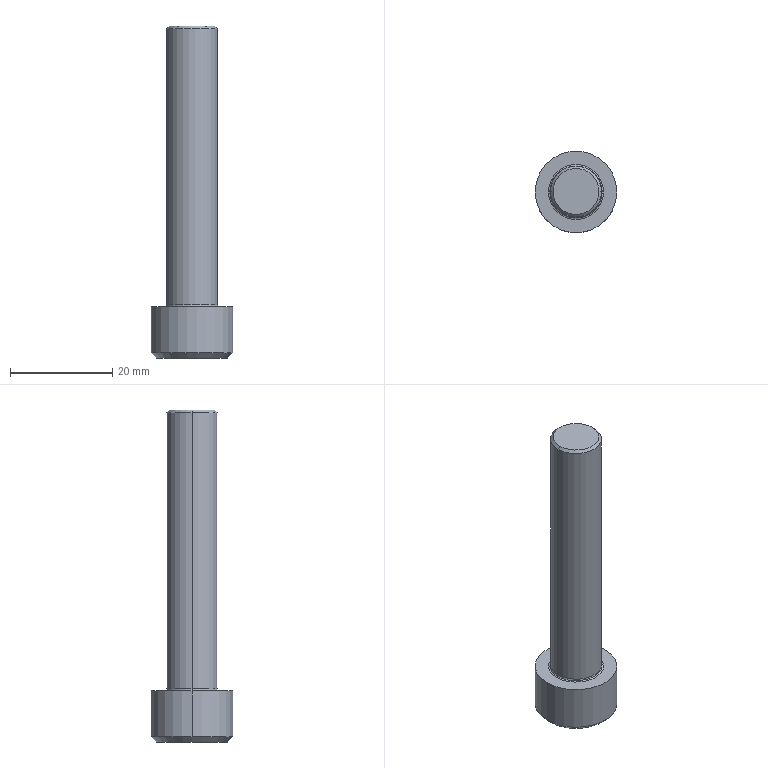Part | Creo | 1 solid | 23 faces | box 16 x 16 x 65 mm | volume 5968 mm3 | plane 9 | cone 6 | cylinder 4 | torus 4 | commonest cylinder face diameters 10 x2 16 x2
STEP:
#1=CARTESIAN_POINT('',(-89.619,220.995,56.));
#2=VERTEX_POINT('',#1);
#3=CARTESIAN_POINT('',(-87.309,224.995,56.));
#4=VERTEX_POINT('',#3);
#5=CARTESIAN_POINT('',(-89.619,220.995,56.));
#6=CARTESIAN_POINT('',(-89.493,221.213,56.073));
#7=CARTESIAN_POINT('',(-89.241,221.65,56.201));
#8=CARTESIAN_POINT('',(-88.855,222.318,56.327));
#9=CARTESIAN_POINT('',(-88.465,222.993,56.372));
#10=CARTESIAN_POINT('',(-88.074,223.671,56.328));
#11=CARTESIAN_POINT('',(-87.689,224.338,56.201));
#12=CARTESIAN_POINT('',(-87.436,224.777,56.073));
#13=CARTESIAN_POINT('',(-87.309,224.995,56.));
#14=B_SPLINE_CURVE_WITH_KNOTS('',3,(#5,#6,#7,#8,#9,#10,#11,#12,#13),.UNSPECIFIED.,.F.,.F.,(4,1,1,1,1,1,4),(0.,0.1667,0.3333,0.5,0.6667,0.8333,1.),.UNSPECIFIED.);
#15=EDGE_CURVE('',#2,#4,#14,.T.);
#16=ORIENTED_EDGE('',*,*,#15,.F.);
#17=CARTESIAN_POINT('',(-85.,220.995,58.667));
#18=VERTEX_POINT('',#17);
#19=CARTESIAN_POINT('',(-85.,220.995,58.667));
#20=DIRECTION('',(-0.866,0.,-0.5));
#21=VECTOR('',#20,5.333);
#22=LINE('',#19,#21);
#23=EDGE_CURVE('',#18,#2,#22,.T.);
#24=ORIENTED_EDGE('',*,*,#23,.F.);
#25=CARTESIAN_POINT('',(-80.381,220.995,56.));
#26=VERTEX_POINT('',#25);
#27=CARTESIAN_POINT('',(-85.,220.995,58.667));
#28=DIRECTION('',(0.866,0.,-0.5));
#29=VECTOR('',#28,5.333);
#30=LINE('',#27,#29);
#31=EDGE_CURVE('',#18,#26,#30,.T.);
#32=ORIENTED_EDGE('',*,*,#31,.T.);
#33=CARTESIAN_POINT('',(-82.691,224.995,56.));
#34=VERTEX_POINT('',#33);
#35=CARTESIAN_POINT('',(-82.691,224.995,56.));
#36=CARTESIAN_POINT('',(-82.565,224.778,56.073));
#37=CARTESIAN_POINT('',(-82.313,224.341,56.201));
#38=CARTESIAN_POINT('',(-81.927,223.672,56.327));
#39=CARTESIAN_POINT('',(-81.537,222.997,56.372));
#40=CARTESIAN_POINT('',(-81.146,222.32,56.328));
#41=CARTESIAN_POINT('',(-80.761,221.652,56.201));
#42=CARTESIAN_POINT('',(-80.507,221.214,56.073));
#43=CARTESIAN_POINT('',(-80.381,220.995,56.));
#44=B_SPLINE_CURVE_WITH_KNOTS('',3,(#35,#36,#37,#38,#39,#40,#41,#42,#43),.UNSPECIFIED.,.F.,.F.,(4,1,1,1,1,1,4),(0.,0.1667,0.3333,0.5,0.6667,0.8333,1.),.UNSPECIFIED.);
#45=EDGE_CURVE('',#34,#26,#44,.T.);
#46=ORIENTED_EDGE('',*,*,#45,.F.);
#47=CARTESIAN_POINT('',(-87.309,224.995,56.));
#48=CARTESIAN_POINT('',(-87.059,224.995,56.072));
#49=CARTESIAN_POINT('',(-86.556,224.995,56.2));
#50=CARTESIAN_POINT('',(-85.782,224.995,56.327));
#51=CARTESIAN_POINT('',(-85.001,224.995,56.372));
#52=CARTESIAN_POINT('',(-84.221,224.995,56.328));
#53=CARTESIAN_POINT('',(-83.447,224.995,56.201));
#54=CARTESIAN_POINT('',(-82.942,224.995,56.073));
#55=CARTESIAN_POINT('',(-82.691,224.995,56.));
#56=B_SPLINE_CURVE_WITH_KNOTS('',3,(#47,#48,#49,#50,#51,#52,#53,#54,#55),.UNSPECIFIED.,.F.,.F.,(4,1,1,1,1,1,4),(0.,0.1667,0.3333,0.5,0.6667,0.8333,1.),.UNSPECIFIED.);
#57=EDGE_CURVE('',#4,#34,#56,.T.);
#58=ORIENTED_EDGE('',*,*,#57,.F.);
#59=EDGE_LOOP('',(#16,#24,#32,#46,#58));
#60=FACE_OUTER_BOUND('',#59,.F.);
#61=CARTESIAN_POINT('',(-85.,220.995,57.307));
#62=DIRECTION('',(0.,0.,-1.));
#63=DIRECTION('',(-1.,0.,0.));
#64=AXIS2_PLACEMENT_3D('',#61,#62,#63);
#65=CONICAL_SURFACE('',#64,2.356,60.);
#66=ADVANCED_FACE('',(#60),#65,.F.);
#67=CARTESIAN_POINT('',(-87.309,224.995,51.));
#68=VERTEX_POINT('',#67);
#69=CARTESIAN_POINT('',(-89.619,220.995,51.));
#70=VERTEX_POINT('',#69);
#71=CARTESIAN_POINT('',(-87.309,224.995,51.));
#72=DIRECTION('',(-0.5,-0.866,0.));
#73=VECTOR('',#72,4.619);
#74=LINE('',#71,#73);
#75=EDGE_CURVE('',#68,#70,#74,.T.);
#76=ORIENTED_EDGE('',*,*,#75,.T.);
#77=CARTESIAN_POINT('',(-89.619,220.995,51.));
#78=DIRECTION('',(0.,0.,1.));
#79=VECTOR('',#78,5.);
#80=LINE('',#77,#79);
#81=EDGE_CURVE('',#70,#2,#80,.T.);
#82=ORIENTED_EDGE('',*,*,#81,.T.);
#83=ORIENTED_EDGE('',*,*,#15,.T.);
#84=CARTESIAN_POINT('',(-87.309,224.995,51.));
#85=DIRECTION('',(0.,0.,1.));
#86=VECTOR('',#85,5.);
#87=LINE('',#84,#86);
#88=EDGE_CURVE('',#68,#4,#87,.T.);
#89=ORIENTED_EDGE('',*,*,#88,.F.);
#90=EDGE_LOOP('',(#76,#82,#83,#89));
#91=FACE_OUTER_BOUND('',#90,.F.);
#92=CARTESIAN_POINT('',(-87.309,224.995,56.));
#93=DIRECTION('',(0.866,-0.5,0.));
#94=DIRECTION('',(-0.5,-0.866,0.));
#95=AXIS2_PLACEMENT_3D('',#92,#93,#94);
#96=PLANE('',#95);
#97=ADVANCED_FACE('',(#91),#96,.T.);
#98=CARTESIAN_POINT('',(-92.,220.995,51.));
#99=VERTEX_POINT('',#98);
#100=CARTESIAN_POINT('',(-78.,220.995,51.));
#101=VERTEX_POINT('',#100);
#102=CARTESIAN_POINT('',(-85.,220.995,51.));
#103=DIRECTION('',(0.,0.,-1.));
#104=DIRECTION('',(-1.,0.,0.));
#105=AXIS2_PLACEMENT_3D('',#102,#103,#104);
#106=CIRCLE('',#105,7.);
#107=EDGE_CURVE('',#99,#101,#106,.T.);
#108=ORIENTED_EDGE('',*,*,#107,.F.);
#109=CARTESIAN_POINT('',(-85.,220.995,51.));
#110=DIRECTION('',(0.,0.,-1.));
#111=DIRECTION('',(1.,0.,0.));
#112=AXIS2_PLACEMENT_3D('',#109,#110,#111);
#113=CIRCLE('',#112,7.);
#114=EDGE_CURVE('',#101,#99,#113,.T.);
#115=ORIENTED_EDGE('',*,*,#114,.F.);
#116=EDGE_LOOP('',(#108,#115));
#117=FACE_OUTER_BOUND('',#116,.F.);
#118=CARTESIAN_POINT('',(-87.309,216.995,51.));
#119=VERTEX_POINT('',#118);
#120=CARTESIAN_POINT('',(-89.619,220.995,51.));
#121=DIRECTION('',(0.5,-0.866,0.));
#122=VECTOR('',#121,4.619);
#123=LINE('',#120,#122);
#124=EDGE_CURVE('',#70,#119,#123,.T.);
#125=ORIENTED_EDGE('',*,*,#124,.F.);
#126=ORIENTED_EDGE('',*,*,#75,.F.);
#127=CARTESIAN_POINT('',(-82.691,224.995,51.));
#128=VERTEX_POINT('',#127);
#129=CARTESIAN_POINT('',(-87.309,224.995,51.));
#130=DIRECTION('',(1.,0.,0.));
#131=VECTOR('',#130,4.619);
#132=LINE('',#129,#131);
#133=EDGE_CURVE('',#68,#128,#132,.T.);
#134=ORIENTED_EDGE('',*,*,#133,.T.);
#135=CARTESIAN_POINT('',(-80.381,220.995,51.));
#136=VERTEX_POINT('',#135);
#137=CARTESIAN_POINT('',(-80.381,220.995,51.));
#138=DIRECTION('',(-0.5,0.866,0.));
#139=VECTOR('',#138,4.619);
#140=LINE('',#137,#139);
#141=EDGE_CURVE('',#136,#128,#140,.T.);
#142=ORIENTED_EDGE('',*,*,#141,.F.);
#143=CARTESIAN_POINT('',(-82.691,216.995,51.));
#144=VERTEX_POINT('',#143);
#145=CARTESIAN_POINT('',(-82.691,216.995,51.));
#146=DIRECTION('',(0.5,0.866,0.));
#147=VECTOR('',#146,4.619);
#148=LINE('',#145,#147);
#149=EDGE_CURVE('',#144,#136,#148,.T.);
#150=ORIENTED_EDGE('',*,*,#149,.F.);
#151=CARTESIAN_POINT('',(-82.691,216.995,51.));
#152=DIRECTION('',(-1.,0.,0.));
#153=VECTOR('',#152,4.619);
#154=LINE('',#151,#153);
#155=EDGE_CURVE('',#144,#119,#154,.T.);
#156=ORIENTED_EDGE('',*,*,#155,.T.);
#157=EDGE_LOOP('',(#125,#126,#134,#142,#150,#156));
#158=FACE_BOUND('',#157,.F.);
#159=CARTESIAN_POINT('',(-85.,220.995,51.));
#160=DIRECTION('',(0.,0.,-1.));
#161=DIRECTION('',(-1.,0.,0.));
#162=AXIS2_PLACEMENT_3D('',#159,#160,#161);
#163=PLANE('',#162);
#164=ADVANCED_FACE('',(#117,#158),#163,.T.);
#165=CARTESIAN_POINT('',(-93.,220.995,52.));
#166=VERTEX_POINT('',#165);
#167=CARTESIAN_POINT('',(-77.,220.995,52.));
#168=VERTEX_POINT('',#167);
#169=CARTESIAN_POINT('',(-85.,220.995,52.));
#170=DIRECTION('',(0.,0.,-1.));
#171=DIRECTION('',(-1.,0.,0.));
#172=AXIS2_PLACEMENT_3D('',#169,#170,#171);
#173=CIRCLE('',#172,8.);
#174=EDGE_CURVE('',#166,#168,#173,.T.);
#175=ORIENTED_EDGE('',*,*,#174,.F.);
#176=CARTESIAN_POINT('',(-92.,220.995,51.));
#177=DIRECTION('',(-0.7071,0.,0.7071));
#178=VECTOR('',#177,1.414);
#179=LINE('',#176,#178);
#180=EDGE_CURVE('',#99,#166,#179,.T.);
#181=ORIENTED_EDGE('',*,*,#180,.F.);
#182=ORIENTED_EDGE('',*,*,#107,.T.);
#183=CARTESIAN_POINT('',(-78.,220.995,51.));
#184=DIRECTION('',(0.7071,0.,0.7071));
#185=VECTOR('',#184,1.414);
#186=LINE('',#183,#185);
#187=EDGE_CURVE('',#101,#168,#186,.T.);
#188=ORIENTED_EDGE('',*,*,#187,.T.);
#189=EDGE_LOOP('',(#175,#181,#182,#188));
#190=FACE_OUTER_BOUND('',#189,.F.);
#191=CARTESIAN_POINT('',(-85.,220.995,51.5));
#192=DIRECTION('',(0.,0.,1.));
#193=DIRECTION('',(1.,0.,0.));
#194=AXIS2_PLACEMENT_3D('',#191,#192,#193);
#195=CONICAL_SURFACE('',#194,7.5,45.);
#196=ADVANCED_FACE('',(#190),#195,.T.);
#197=ORIENTED_EDGE('',*,*,#174,.T.);
#198=CARTESIAN_POINT('',(-77.,220.995,61.));
#199=VERTEX_POINT('',#198);
#200=CARTESIAN_POINT('',(-77.,220.995,61.));
#201=DIRECTION('',(0.,0.,-1.));
#202=VECTOR('',#201,9.);
#203=LINE('',#200,#202);
#204=EDGE_CURVE('',#199,#168,#203,.T.);
#205=ORIENTED_EDGE('',*,*,#204,.F.);
#206=CARTESIAN_POINT('',(-93.,220.995,61.));
#207=VERTEX_POINT('',#206);
#208=CARTESIAN_POINT('',(-85.,220.995,61.));
#209=DIRECTION('',(0.,0.,1.));
#210=DIRECTION('',(1.,0.,0.));
#211=AXIS2_PLACEMENT_3D('',#208,#209,#210);
#212=CIRCLE('',#211,8.);
#213=EDGE_CURVE('',#199,#207,#212,.T.);
#214=ORIENTED_EDGE('',*,*,#213,.T.);
#215=CARTESIAN_POINT('',(-93.,220.995,61.));
#216=DIRECTION('',(0.,0.,-1.));
#217=VECTOR('',#216,9.);
#218=LINE('',#215,#217);
#219=EDGE_CURVE('',#207,#166,#218,.T.);
#220=ORIENTED_EDGE('',*,*,#219,.T.);
#221=EDGE_LOOP('',(#197,#205,#214,#220));
#222=FACE_OUTER_BOUND('',#221,.F.);
#223=CARTESIAN_POINT('',(-85.,220.995,61.));
#224=DIRECTION('',(0.,0.,-1.));
#225=DIRECTION('',(-1.,0.,0.));
#226=AXIS2_PLACEMENT_3D('',#223,#224,#225);
#227=CYLINDRICAL_SURFACE('',#226,8.);
#228=ADVANCED_FACE('',(#222),#227,.T.);
#229=CARTESIAN_POINT('',(-85.,220.995,52.));
#230=DIRECTION('',(0.,0.,-1.));
#231=DIRECTION('',(1.,0.,0.));
#232=AXIS2_PLACEMENT_3D('',#229,#230,#231);
#233=CIRCLE('',#232,8.);
#234=EDGE_CURVE('',#168,#166,#233,.T.);
#235=ORIENTED_EDGE('',*,*,#234,.T.);
#236=ORIENTED_EDGE('',*,*,#219,.F.);
#237=CARTESIAN_POINT('',(-85.,220.995,61.));
#238=DIRECTION('',(0.,0.,1.));
#239=DIRECTION('',(-1.,0.,0.));
#240=AXIS2_PLACEMENT_3D('',#237,#238,#239);
#241=CIRCLE('',#240,8.);
#242=EDGE_CURVE('',#207,#199,#241,.T.);
#243=ORIENTED_EDGE('',*,*,#242,.T.);
#244=ORIENTED_EDGE('',*,*,#204,.T.);
#245=EDGE_LOOP('',(#235,#236,#243,#244));
#246=FACE_OUTER_BOUND('',#245,.F.);
#247=CARTESIAN_POINT('',(-85.,220.995,61.));
#248=DIRECTION('',(0.,0.,-1.));
#249=DIRECTION('',(-1.,0.,0.));
#250=AXIS2_PLACEMENT_3D('',#247,#248,#249);
#251=CYLINDRICAL_SURFACE('',#250,8.);
#252=ADVANCED_FACE('',(#246),#251,.T.);
#253=ORIENTED_EDGE('',*,*,#234,.F.);
#254=ORIENTED_EDGE('',*,*,#187,.F.);
#255=ORIENTED_EDGE('',*,*,#114,.T.);
#256=ORIENTED_EDGE('',*,*,#180,.T.);
#257=EDGE_LOOP('',(#253,#254,#255,#256));
#258=FACE_OUTER_BOUND('',#257,.F.);
#259=CARTESIAN_POINT('',(-85.,220.995,51.5));
#260=DIRECTION('',(0.,0.,1.));
#261=DIRECTION('',(1.,0.,0.));
#262=AXIS2_PLACEMENT_3D('',#259,#260,#261);
#263=CONICAL_SURFACE('',#262,7.5,45.);
#264=ADVANCED_FACE('',(#258),#263,.T.);
#265=ORIENTED_EDGE('',*,*,#242,.F.);
#266=ORIENTED_EDGE('',*,*,#213,.F.);
#267=EDGE_LOOP('',(#265,#266));
#268=FACE_OUTER_BOUND('',#267,.F.);
#269=CARTESIAN_POINT('',(-90.4,220.995,61.));
#270=VERTEX_POINT('',#269);
#271=CARTESIAN_POINT('',(-79.6,220.995,61.));
#272=VERTEX_POINT('',#271);
#273=CARTESIAN_POINT('',(-85.,220.995,61.));
#274=DIRECTION('',(0.,0.,-1.));
#275=DIRECTION('',(-1.,0.,0.));
#276=AXIS2_PLACEMENT_3D('',#273,#274,#275);
#277=CIRCLE('',#276,5.4);
#278=EDGE_CURVE('',#270,#272,#277,.T.);
#279=ORIENTED_EDGE('',*,*,#278,.F.);
#280=CARTESIAN_POINT('',(-85.,220.995,61.));
#281=DIRECTION('',(0.,0.,-1.));
#282=DIRECTION('',(1.,0.,0.));
#283=AXIS2_PLACEMENT_3D('',#280,#281,#282);
#284=CIRCLE('',#283,5.4);
#285=EDGE_CURVE('',#272,#270,#284,.T.);
#286=ORIENTED_EDGE('',*,*,#285,.F.);
#287=EDGE_LOOP('',(#279,#286));
#288=FACE_BOUND('',#287,.F.);
#289=CARTESIAN_POINT('',(-85.,220.995,61.));
#290=DIRECTION('',(0.,0.,-1.));
#291=DIRECTION('',(-1.,0.,0.));
#292=AXIS2_PLACEMENT_3D('',#289,#290,#291);
#293=PLANE('',#292);
#294=ADVANCED_FACE('',(#268,#288),#293,.F.);
#295=ORIENTED_EDGE('',*,*,#278,.T.);
#296=CARTESIAN_POINT('',(-79.883,220.995,61.117));
#297=VERTEX_POINT('',#296);
#298=CARTESIAN_POINT('',(-79.6,220.995,61.4));
#299=DIRECTION('',(0.,1.,0.));
#300=DIRECTION('',(0.,0.,-1.));
#301=AXIS2_PLACEMENT_3D('',#298,#299,#300);
#302=CIRCLE('',#301,0.4);
#303=EDGE_CURVE('',#272,#297,#302,.T.);
#304=ORIENTED_EDGE('',*,*,#303,.T.);
#305=CARTESIAN_POINT('',(-90.117,220.995,61.117));
#306=VERTEX_POINT('',#305);
#307=CARTESIAN_POINT('',(-85.,220.995,61.117));
#308=DIRECTION('',(0.,0.,-1.));
#309=DIRECTION('',(-1.,0.,0.));
#310=AXIS2_PLACEMENT_3D('',#307,#308,#309);
#311=CIRCLE('',#310,5.117);
#312=EDGE_CURVE('',#306,#297,#311,.T.);
#313=ORIENTED_EDGE('',*,*,#312,.F.);
#314=CARTESIAN_POINT('',(-90.4,220.995,61.4));
#315=DIRECTION('',(0.,-1.,0.));
#316=DIRECTION('',(0.,0.,-1.));
#317=AXIS2_PLACEMENT_3D('',#314,#315,#316);
#318=CIRCLE('',#317,0.4);
#319=EDGE_CURVE('',#270,#306,#318,.T.);
#320=ORIENTED_EDGE('',*,*,#319,.F.);
#321=EDGE_LOOP('',(#295,#304,#313,#320));
#322=FACE_OUTER_BOUND('',#321,.F.);
#323=CARTESIAN_POINT('',(-85.,220.995,61.4));
#324=DIRECTION('',(0.,0.,-1.));
#325=DIRECTION('',(-1.,0.,0.));
#326=AXIS2_PLACEMENT_3D('',#323,#324,#325);
#327=TOROIDAL_SURFACE('',#326,5.4,0.4);
#328=ADVANCED_FACE('',(#322),#327,.F.);
#329=ORIENTED_EDGE('',*,*,#285,.T.);
#330=ORIENTED_EDGE('',*,*,#319,.T.);
#331=CARTESIAN_POINT('',(-85.,220.995,61.117));
#332=DIRECTION('',(0.,0.,-1.));
#333=DIRECTION('',(1.,0.,0.));
#334=AXIS2_PLACEMENT_3D('',#331,#332,#333);
#335=CIRCLE('',#334,5.117);
#336=EDGE_CURVE('',#297,#306,#335,.T.);
#337=ORIENTED_EDGE('',*,*,#336,.F.);
#338=ORIENTED_EDGE('',*,*,#303,.F.);
#339=EDGE_LOOP('',(#329,#330,#337,#338));
#340=FACE_OUTER_BOUND('',#339,.F.);
#341=CARTESIAN_POINT('',(-85.,220.995,61.4));
#342=DIRECTION('',(0.,0.,-1.));
#343=DIRECTION('',(-1.,0.,0.));
#344=AXIS2_PLACEMENT_3D('',#341,#342,#343);
#345=TOROIDAL_SURFACE('',#344,5.4,0.4);
#346=ADVANCED_FACE('',(#340),#345,.F.);
#347=CARTESIAN_POINT('',(-80.,220.995,61.4));
#348=VERTEX_POINT('',#347);
#349=CARTESIAN_POINT('',(-90.,220.995,61.4));
#350=VERTEX_POINT('',#349);
#351=CARTESIAN_POINT('',(-85.,220.995,61.4));
#352=DIRECTION('',(0.,0.,-1.));
#353=DIRECTION('',(1.,0.,0.));
#354=AXIS2_PLACEMENT_3D('',#351,#352,#353);
#355=CIRCLE('',#354,5.);
#356=EDGE_CURVE('',#348,#350,#355,.T.);
#357=ORIENTED_EDGE('',*,*,#356,.F.);
#358=CARTESIAN_POINT('',(-79.6,220.995,61.4));
#359=DIRECTION('',(0.,1.,0.));
#360=DIRECTION('',(-0.7071,0.,-0.7071));
#361=AXIS2_PLACEMENT_3D('',#358,#359,#360);
#362=CIRCLE('',#361,0.4);
#363=EDGE_CURVE('',#297,#348,#362,.T.);
#364=ORIENTED_EDGE('',*,*,#363,.F.);
#365=ORIENTED_EDGE('',*,*,#336,.T.);
#366=CARTESIAN_POINT('',(-90.4,220.995,61.4));
#367=DIRECTION('',(0.,-1.,0.));
#368=DIRECTION('',(0.7071,0.,-0.7071));
#369=AXIS2_PLACEMENT_3D('',#366,#367,#368);
#370=CIRCLE('',#369,0.4);
#371=EDGE_CURVE('',#306,#350,#370,.T.);
#372=ORIENTED_EDGE('',*,*,#371,.T.);
#373=EDGE_LOOP('',(#357,#364,#365,#372));
#374=FACE_OUTER_BOUND('',#373,.F.);
#375=CARTESIAN_POINT('',(-85.,220.995,61.4));
#376=DIRECTION('',(0.,0.,-1.));
#377=DIRECTION('',(-1.,0.,0.));
#378=AXIS2_PLACEMENT_3D('',#375,#376,#377);
#379=TOROIDAL_SURFACE('',#378,5.4,0.4);
#380=ADVANCED_FACE('',(#374),#379,.F.);
#381=CARTESIAN_POINT('',(-90.,220.995,115.5));
#382=VERTEX_POINT('',#381);
#383=CARTESIAN_POINT('',(-80.,220.995,115.5));
#384=VERTEX_POINT('',#383);
#385=CARTESIAN_POINT('',(-85.,220.995,115.5));
#386=DIRECTION('',(0.,0.,1.));
#387=DIRECTION('',(-1.,0.,0.));
#388=AXIS2_PLACEMENT_3D('',#385,#386,#387);
#389=CIRCLE('',#388,5.);
#390=EDGE_CURVE('',#382,#384,#389,.T.);
#391=ORIENTED_EDGE('',*,*,#390,.T.);
#392=CARTESIAN_POINT('',(-80.,220.995,115.5));
#393=DIRECTION('',(0.,0.,-1.));
#394=VECTOR('',#393,54.1);
#395=LINE('',#392,#394);
#396=EDGE_CURVE('',#384,#348,#395,.T.);
#397=ORIENTED_EDGE('',*,*,#396,.T.);
#398=ORIENTED_EDGE('',*,*,#356,.T.);
#399=CARTESIAN_POINT('',(-90.,220.995,115.5));
#400=DIRECTION('',(0.,0.,-1.));
#401=VECTOR('',#400,54.1);
#402=LINE('',#399,#401);
#403=EDGE_CURVE('',#382,#350,#402,.T.);
#404=ORIENTED_EDGE('',*,*,#403,.F.);
#405=EDGE_LOOP('',(#391,#397,#398,#404));
#406=FACE_OUTER_BOUND('',#405,.F.);
#407=CARTESIAN_POINT('',(-85.,220.995,116.));
#408=DIRECTION('',(0.,0.,-1.));
#409=DIRECTION('',(-1.,0.,0.));
#410=AXIS2_PLACEMENT_3D('',#407,#408,#409);
#411=CYLINDRICAL_SURFACE('',#410,5.);
#412=ADVANCED_FACE('',(#406),#411,.T.);
#413=CARTESIAN_POINT('',(-89.5,220.995,116.));
#414=VERTEX_POINT('',#413);
#415=CARTESIAN_POINT('',(-80.5,220.995,116.));
#416=VERTEX_POINT('',#415);
#417=CARTESIAN_POINT('',(-85.,220.995,116.));
#418=DIRECTION('',(0.,0.,1.));
#419=DIRECTION('',(-1.,0.,0.));
#420=AXIS2_PLACEMENT_3D('',#417,#418,#419);
#421=CIRCLE('',#420,4.5);
#422=EDGE_CURVE('',#414,#416,#421,.T.);
#423=ORIENTED_EDGE('',*,*,#422,.T.);
#424=CARTESIAN_POINT('',(-80.5,220.995,116.));
#425=DIRECTION('',(0.7071,0.,-0.7071));
#426=VECTOR('',#425,0.7071);
#427=LINE('',#424,#426);
#428=EDGE_CURVE('',#416,#384,#427,.T.);
#429=ORIENTED_EDGE('',*,*,#428,.T.);
#430=ORIENTED_EDGE('',*,*,#390,.F.);
#431=CARTESIAN_POINT('',(-89.5,220.995,116.));
#432=DIRECTION('',(-0.7071,0.,-0.7071));
#433=VECTOR('',#432,0.7071);
#434=LINE('',#431,#433);
#435=EDGE_CURVE('',#414,#382,#434,.T.);
#436=ORIENTED_EDGE('',*,*,#435,.F.);
#437=EDGE_LOOP('',(#423,#429,#430,#436));
#438=FACE_OUTER_BOUND('',#437,.F.);
#439=CARTESIAN_POINT('',(-85.,220.995,115.75));
#440=DIRECTION('',(0.,0.,-1.));
#441=DIRECTION('',(-1.,0.,0.));
#442=AXIS2_PLACEMENT_3D('',#439,#440,#441);
#443=CONICAL_SURFACE('',#442,4.75,45.);
#444=ADVANCED_FACE('',(#438),#443,.T.);
#445=ORIENTED_EDGE('',*,*,#422,.F.);
#446=CARTESIAN_POINT('',(-85.,220.995,116.));
#447=DIRECTION('',(0.,0.,1.));
#448=DIRECTION('',(1.,0.,0.));
#449=AXIS2_PLACEMENT_3D('',#446,#447,#448);
#450=CIRCLE('',#449,4.5);
#451=EDGE_CURVE('',#416,#414,#450,.T.);
#452=ORIENTED_EDGE('',*,*,#451,.F.);
#453=EDGE_LOOP('',(#445,#452));
#454=FACE_OUTER_BOUND('',#453,.F.);
#455=CARTESIAN_POINT('',(-85.,220.995,116.));
#456=DIRECTION('',(0.,0.,-1.));
#457=DIRECTION('',(-1.,0.,0.));
#458=AXIS2_PLACEMENT_3D('',#455,#456,#457);
#459=PLANE('',#458);
#460=ADVANCED_FACE('',(#454),#459,.F.);
#461=ORIENTED_EDGE('',*,*,#451,.T.);
#462=ORIENTED_EDGE('',*,*,#435,.T.);
#463=CARTESIAN_POINT('',(-85.,220.995,115.5));
#464=DIRECTION('',(0.,0.,1.));
#465=DIRECTION('',(1.,0.,0.));
#466=AXIS2_PLACEMENT_3D('',#463,#464,#465);
#467=CIRCLE('',#466,5.);
#468=EDGE_CURVE('',#384,#382,#467,.T.);
#469=ORIENTED_EDGE('',*,*,#468,.F.);
#470=ORIENTED_EDGE('',*,*,#428,.F.);
#471=EDGE_LOOP('',(#461,#462,#469,#470));
#472=FACE_OUTER_BOUND('',#471,.F.);
#473=CARTESIAN_POINT('',(-85.,220.995,115.75));
#474=DIRECTION('',(0.,0.,-1.));
#475=DIRECTION('',(-1.,0.,0.));
#476=AXIS2_PLACEMENT_3D('',#473,#474,#475);
#477=CONICAL_SURFACE('',#476,4.75,45.);
#478=ADVANCED_FACE('',(#472),#477,.T.);
#479=ORIENTED_EDGE('',*,*,#468,.T.);
#480=ORIENTED_EDGE('',*,*,#403,.T.);
#481=CARTESIAN_POINT('',(-85.,220.995,61.4));
#482=DIRECTION('',(0.,0.,-1.));
#483=DIRECTION('',(-1.,0.,0.));
#484=AXIS2_PLACEMENT_3D('',#481,#482,#483);
#485=CIRCLE('',#484,5.);
#486=EDGE_CURVE('',#350,#348,#485,.T.);
#487=ORIENTED_EDGE('',*,*,#486,.T.);
#488=ORIENTED_EDGE('',*,*,#396,.F.);
#489=EDGE_LOOP('',(#479,#480,#487,#488));
#490=FACE_OUTER_BOUND('',#489,.F.);
#491=CARTESIAN_POINT('',(-85.,220.995,116.));
#492=DIRECTION('',(0.,0.,-1.));
#493=DIRECTION('',(-1.,0.,0.));
#494=AXIS2_PLACEMENT_3D('',#491,#492,#493);
#495=CYLINDRICAL_SURFACE('',#494,5.);
#496=ADVANCED_FACE('',(#490),#495,.T.);
#497=ORIENTED_EDGE('',*,*,#486,.F.);
#498=ORIENTED_EDGE('',*,*,#371,.F.);
#499=ORIENTED_EDGE('',*,*,#312,.T.);
#500=ORIENTED_EDGE('',*,*,#363,.T.);
#501=EDGE_LOOP('',(#497,#498,#499,#500));
#502=FACE_OUTER_BOUND('',#501,.F.);
#503=CARTESIAN_POINT('',(-85.,220.995,61.4));
#504=DIRECTION('',(0.,0.,-1.));
#505=DIRECTION('',(-1.,0.,0.));
#506=AXIS2_PLACEMENT_3D('',#503,#504,#505);
#507=TOROIDAL_SURFACE('',#506,5.4,0.4);
#508=ADVANCED_FACE('',(#502),#507,.F.);
#509=ORIENTED_EDGE('',*,*,#124,.T.);
#510=CARTESIAN_POINT('',(-87.309,216.995,56.));
#511=VERTEX_POINT('',#510);
#512=CARTESIAN_POINT('',(-87.309,216.995,51.));
#513=DIRECTION('',(0.,0.,1.));
#514=VECTOR('',#513,5.);
#515=LINE('',#512,#514);
#516=EDGE_CURVE('',#119,#511,#515,.T.);
#517=ORIENTED_EDGE('',*,*,#516,.T.);
#518=CARTESIAN_POINT('',(-87.309,216.995,56.));
#519=CARTESIAN_POINT('',(-87.435,217.213,56.073));
#520=CARTESIAN_POINT('',(-87.687,217.65,56.201));
#521=CARTESIAN_POINT('',(-88.073,218.318,56.327));
#522=CARTESIAN_POINT('',(-88.463,218.993,56.372));
#523=CARTESIAN_POINT('',(-88.854,219.671,56.328));
#524=CARTESIAN_POINT('',(-89.239,220.338,56.201));
#525=CARTESIAN_POINT('',(-89.493,220.777,56.073));
#526=CARTESIAN_POINT('',(-89.619,220.995,56.));
#527=B_SPLINE_CURVE_WITH_KNOTS('',3,(#518,#519,#520,#521,#522,#523,#524,#525,#526),.UNSPECIFIED.,.F.,.F.,(4,1,1,1,1,1,4),(0.,0.1667,0.3333,0.5,0.6667,0.8333,1.),.UNSPECIFIED.);
#528=EDGE_CURVE('',#511,#2,#527,.T.);
#529=ORIENTED_EDGE('',*,*,#528,.T.);
#530=ORIENTED_EDGE('',*,*,#81,.F.);
#531=EDGE_LOOP('',(#509,#517,#529,#530));
#532=FACE_OUTER_BOUND('',#531,.F.);
#533=CARTESIAN_POINT('',(-89.619,220.995,56.));
#534=DIRECTION('',(0.866,0.5,0.));
#535=DIRECTION('',(0.5,-0.866,0.));
#536=AXIS2_PLACEMENT_3D('',#533,#534,#535);
#537=PLANE('',#536);
#538=ADVANCED_FACE('',(#532),#537,.T.);
#539=ORIENTED_EDGE('',*,*,#155,.F.);
#540=CARTESIAN_POINT('',(-82.691,216.995,56.));
#541=VERTEX_POINT('',#540);
#542=CARTESIAN_POINT('',(-82.691,216.995,51.));
#543=DIRECTION('',(0.,0.,1.));
#544=VECTOR('',#543,5.);
#545=LINE('',#542,#544);
#546=EDGE_CURVE('',#144,#541,#545,.T.);
#547=ORIENTED_EDGE('',*,*,#546,.T.);
#548=CARTESIAN_POINT('',(-82.691,216.995,56.));
#549=CARTESIAN_POINT('',(-82.942,216.995,56.073));
#550=CARTESIAN_POINT('',(-83.447,216.995,56.201));
#551=CARTESIAN_POINT('',(-84.221,216.995,56.328));
#552=CARTESIAN_POINT('',(-85.001,216.995,56.372));
#553=CARTESIAN_POINT('',(-85.782,216.995,56.327));
#554=CARTESIAN_POINT('',(-86.556,216.995,56.2));
#555=CARTESIAN_POINT('',(-87.059,216.995,56.072));
#556=CARTESIAN_POINT('',(-87.309,216.995,56.));
#557=B_SPLINE_CURVE_WITH_KNOTS('',3,(#548,#549,#550,#551,#552,#553,#554,#555,#556),.UNSPECIFIED.,.F.,.F.,(4,1,1,1,1,1,4),(0.,0.1667,0.3333,0.5,0.6667,0.8333,1.),.UNSPECIFIED.);
#558=EDGE_CURVE('',#541,#511,#557,.T.);
#559=ORIENTED_EDGE('',*,*,#558,.T.);
#560=ORIENTED_EDGE('',*,*,#516,.F.);
#561=EDGE_LOOP('',(#539,#547,#559,#560));
#562=FACE_OUTER_BOUND('',#561,.F.);
#563=CARTESIAN_POINT('',(-87.309,216.995,56.));
#564=DIRECTION('',(0.,1.,0.));
#565=DIRECTION('',(0.,0.,-1.));
#566=AXIS2_PLACEMENT_3D('',#563,#564,#565);
#567=PLANE('',#566);
#568=ADVANCED_FACE('',(#562),#567,.T.);
#569=ORIENTED_EDGE('',*,*,#149,.T.);
#570=CARTESIAN_POINT('',(-80.381,220.995,51.));
#571=DIRECTION('',(0.,0.,1.));
#572=VECTOR('',#571,5.);
#573=LINE('',#570,#572);
#574=EDGE_CURVE('',#136,#26,#573,.T.);
#575=ORIENTED_EDGE('',*,*,#574,.T.);
#576=CARTESIAN_POINT('',(-80.381,220.995,56.));
#577=CARTESIAN_POINT('',(-80.507,220.777,56.073));
#578=CARTESIAN_POINT('',(-80.761,220.338,56.201));
#579=CARTESIAN_POINT('',(-81.146,219.671,56.328));
#580=CARTESIAN_POINT('',(-81.537,218.993,56.372));
#581=CARTESIAN_POINT('',(-81.927,218.318,56.327));
#582=CARTESIAN_POINT('',(-82.313,217.65,56.201));
#583=CARTESIAN_POINT('',(-82.565,217.213,56.073));
#584=CARTESIAN_POINT('',(-82.691,216.995,56.));
#585=B_SPLINE_CURVE_WITH_KNOTS('',3,(#576,#577,#578,#579,#580,#581,#582,#583,#584),.UNSPECIFIED.,.F.,.F.,(4,1,1,1,1,1,4),(0.,0.1667,0.3333,0.5,0.6667,0.8333,1.),.UNSPECIFIED.);
#586=EDGE_CURVE('',#26,#541,#585,.T.);
#587=ORIENTED_EDGE('',*,*,#586,.T.);
#588=ORIENTED_EDGE('',*,*,#546,.F.);
#589=EDGE_LOOP('',(#569,#575,#587,#588));
#590=FACE_OUTER_BOUND('',#589,.F.);
#591=CARTESIAN_POINT('',(-82.691,216.995,56.));
#592=DIRECTION('',(-0.866,0.5,0.));
#593=DIRECTION('',(0.5,0.866,0.));
#594=AXIS2_PLACEMENT_3D('',#591,#592,#593);
#595=PLANE('',#594);
#596=ADVANCED_FACE('',(#590),#595,.T.);
#597=ORIENTED_EDGE('',*,*,#141,.T.);
#598=CARTESIAN_POINT('',(-82.691,224.995,51.));
#599=DIRECTION('',(0.,0.,1.));
#600=VECTOR('',#599,5.);
#601=LINE('',#598,#600);
#602=EDGE_CURVE('',#128,#34,#601,.T.);
#603=ORIENTED_EDGE('',*,*,#602,.T.);
#604=ORIENTED_EDGE('',*,*,#45,.T.);
#605=ORIENTED_EDGE('',*,*,#574,.F.);
#606=EDGE_LOOP('',(#597,#603,#604,#605));
#607=FACE_OUTER_BOUND('',#606,.F.);
#608=CARTESIAN_POINT('',(-80.381,220.995,56.));
#609=DIRECTION('',(-0.866,-0.5,0.));
#610=DIRECTION('',(-0.5,0.866,0.));
#611=AXIS2_PLACEMENT_3D('',#608,#609,#610);
#612=PLANE('',#611);
#613=ADVANCED_FACE('',(#607),#612,.T.);
#614=ORIENTED_EDGE('',*,*,#133,.F.);
#615=ORIENTED_EDGE('',*,*,#88,.T.);
#616=ORIENTED_EDGE('',*,*,#57,.T.);
#617=ORIENTED_EDGE('',*,*,#602,.F.);
#618=EDGE_LOOP('',(#614,#615,#616,#617));
#619=FACE_OUTER_BOUND('',#618,.F.);
#620=CARTESIAN_POINT('',(-82.691,224.995,56.));
#621=DIRECTION('',(0.,-1.,0.));
#622=DIRECTION('',(0.,0.,1.));
#623=AXIS2_PLACEMENT_3D('',#620,#621,#622);
#624=PLANE('',#623);
#625=ADVANCED_FACE('',(#619),#624,.T.);
#626=ORIENTED_EDGE('',*,*,#586,.F.);
#627=ORIENTED_EDGE('',*,*,#31,.F.);
#628=ORIENTED_EDGE('',*,*,#23,.T.);
#629=ORIENTED_EDGE('',*,*,#528,.F.);
#630=ORIENTED_EDGE('',*,*,#558,.F.);
#631=EDGE_LOOP('',(#626,#627,#628,#629,#630));
#632=FACE_OUTER_BOUND('',#631,.F.);
#633=CARTESIAN_POINT('',(-85.,220.995,57.307));
#634=DIRECTION('',(0.,0.,-1.));
#635=DIRECTION('',(-1.,0.,0.));
#636=AXIS2_PLACEMENT_3D('',#633,#634,#635);
#637=CONICAL_SURFACE('',#636,2.356,60.);
#638=ADVANCED_FACE('',(#632),#637,.F.);
#639=CLOSED_SHELL('',(#66,#97,#164,#196,#228,#252,#264,#294,#328,#346,#380,#412,#444,#460,#478,#496,#508,#538,#568,#596,#613,#625,#638));
#640=MANIFOLD_SOLID_BREP('',#639);
#641=(LENGTH_UNIT()NAMED_UNIT(*)SI_UNIT(.MILLI.,.METRE.));
#642=UNCERTAINTY_MEASURE_WITH_UNIT(LENGTH_MEASURE(0.006882),#641,'','');
#643=(NAMED_UNIT(*)PLANE_ANGLE_UNIT()SI_UNIT($,.RADIAN.));
#644=PLANE_ANGLE_MEASURE_WITH_UNIT(PLANE_ANGLE_MEASURE(0.01745),#643);
#645=(CONVERSION_BASED_UNIT('DEGREE',#644)NAMED_UNIT(*)PLANE_ANGLE_UNIT());
#646=(NAMED_UNIT(*)SI_UNIT($,.STERADIAN.)SOLID_ANGLE_UNIT());
#647=(GEOMETRIC_REPRESENTATION_CONTEXT(3)GLOBAL_UNCERTAINTY_ASSIGNED_CONTEXT((#642))GLOBAL_UNIT_ASSIGNED_CONTEXT((#641,#645,#646))REPRESENTATION_CONTEXT('',''));
#648=ADVANCED_BREP_SHAPE_REPRESENTATION('',(#640),#647);